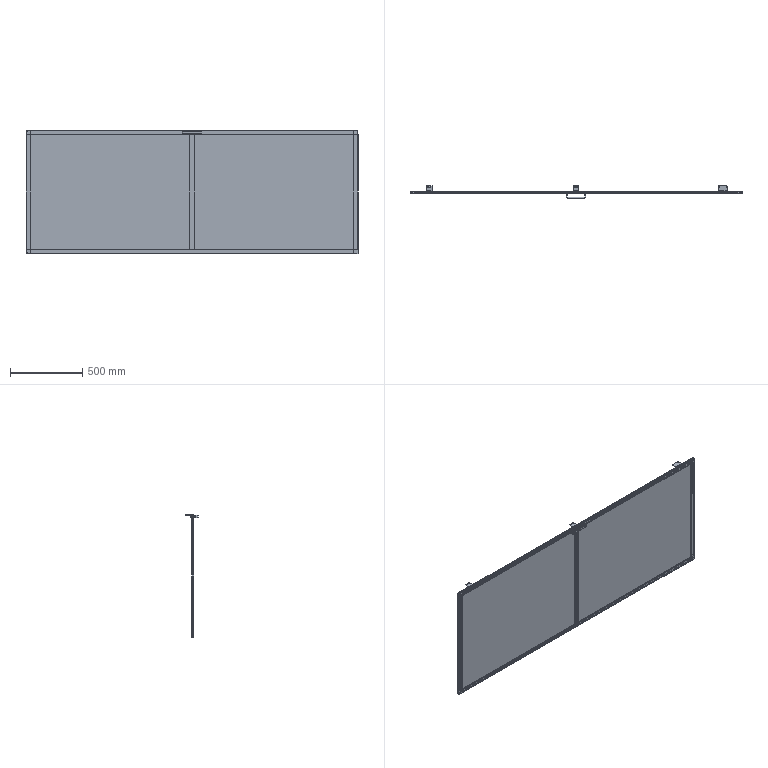Part | 39 solids | 1337 faces | box 2296 x 84 x 851 mm | volume 10757622 mm3 | plane 792 | cylinder 369 | cone 120 | spline 56 | commonest cylinder face diameters 5 x67 11 x52 1 x42 4.5 x40 3.3 x28 2 x20